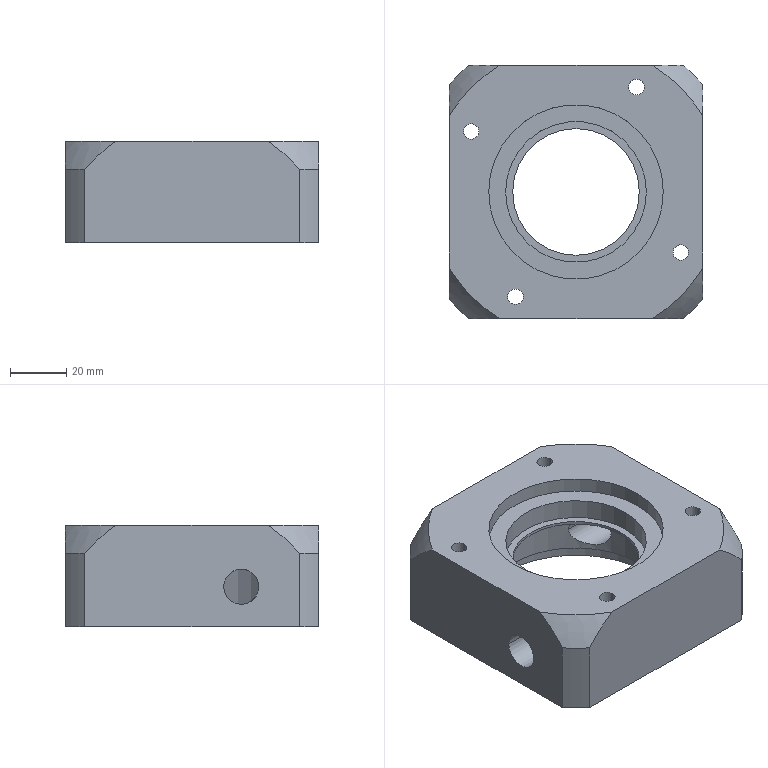Part | SolidWorks | features BaseBody 1 | 1 solid | 68 faces | box 90 x 90 x 36 mm | volume 168447 mm3 | cylinder 42 | plane 14 | cone 8 | torus 4 | commonest cylinder face diameters 4.2 x8 5.5 x8 9.9 x8 12.5 x4 62 x4 118 x4